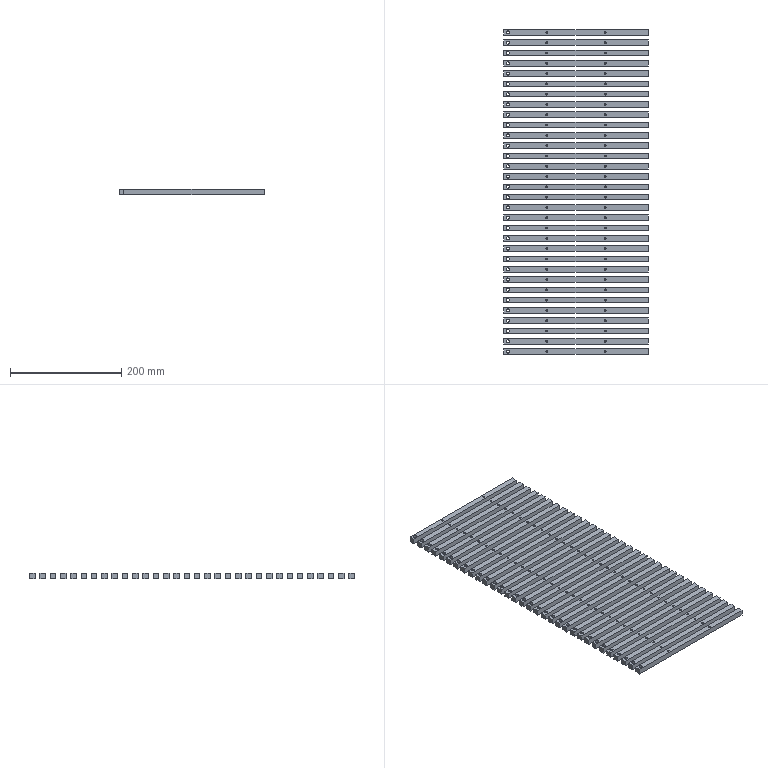CAM job | NX | 3-axis milling, drilling | part box 260 x 583.5 x 10 mm | stock box 264 x 587.5 x 11 mm
Tools:
number,name,description,diameter,corner_radius,flute_length,length,flutes
1,D63,Milling Tool-5 Parameters,63.0,0.0,50.0,75.0,2
7,D6A45,Milling Tool-5 Parameters,6.0,0.0,3.0,3.0,2
13,3.3ZT,Drilling Tool,3.3,0.0,35.0,50.0,2
17,M4,Milling Tool-5 Parameters,3.3,0.0,30.0,30.0,4
12,5.5ZT,Drilling Tool,5.5,0.0,35.0,50.0,2
6,D6,Milling Tool-5 Parameters,6.0,0.0,50.0,75.0,2
Operations:
program,operation,operation_type,tool,method,geometry_group,spindle_rpm,surface_speed,feed_per_tooth,feed_cut,feed_plunge,cut_length_mm,path_length_mm,cut_time_min,machine_time_min
1-590-263-10毛胚AB胶,FLOOR_WALL,VolumeBased25DMillingOperation,D63,METHOD,A,6500.0,1286.0,0.0962,1250.0,100.0,6105.297,6159.297,4.884,4.89
1-590-263-10毛胚AB胶,DRILLING_COPY_1,Operation,D6A45,METHOD,A,3000.0,56.0,0.0333,200.0,0.0,489.6,3242.282,2.448,2.723
1-590-263-10毛胚AB胶,DRILLING_COPY_1_COPY_COPY_COPY_COPY_COPY,Operation,3.3ZT,METHOD,A,2000.0,20.0,0.0375,150.0,0.0,991.451,3498.928,6.61,6.86
1-590-263-10毛胚AB胶,DRILLING_COPY_1_COPY_COPY_COPY_COPY_COPY_COPY_1,Operation,M4,METHOD,A,200.0,2.0,0.175,140.0,0.0,864.0,3244.026,6.171,6.409
1-590-263-10毛胚AB胶,DRILLING_COPY_1_COPY_COPY_1_COPY_1,Operation,5.5ZT,METHOD,A,2000.0,18.0,0.03,120.0,0.0,516.876,1767.743,4.307,4.432
1-590-263-10毛胚AB胶,ZLEVEL_PROFILE,ZLevelMilling,D6,METHOD,A,7000.0,219.0,0.2143,3000.0,1000.0,431604.187,437769.328,144.639,145.256
1-590-263-10毛胚AB胶,ZLEVEL_PROFILE_COPY_1_COPY_COPY_COPY_COPY_2_COPY,ZLevelMilling,D6A45,METHOD,A,7000.0,131.0,0.0714,1000.0,1000.0,18417.68,44585.247,18.418,21.034
1-590-263-10毛胚AB胶,ZLEVEL_PROFILE_COPY_1_1,ZLevelMilling,D6,METHOD,A,7000.0,219.0,0.0714,1000.0,1000.0,54930.997,66270.677,54.931,56.065